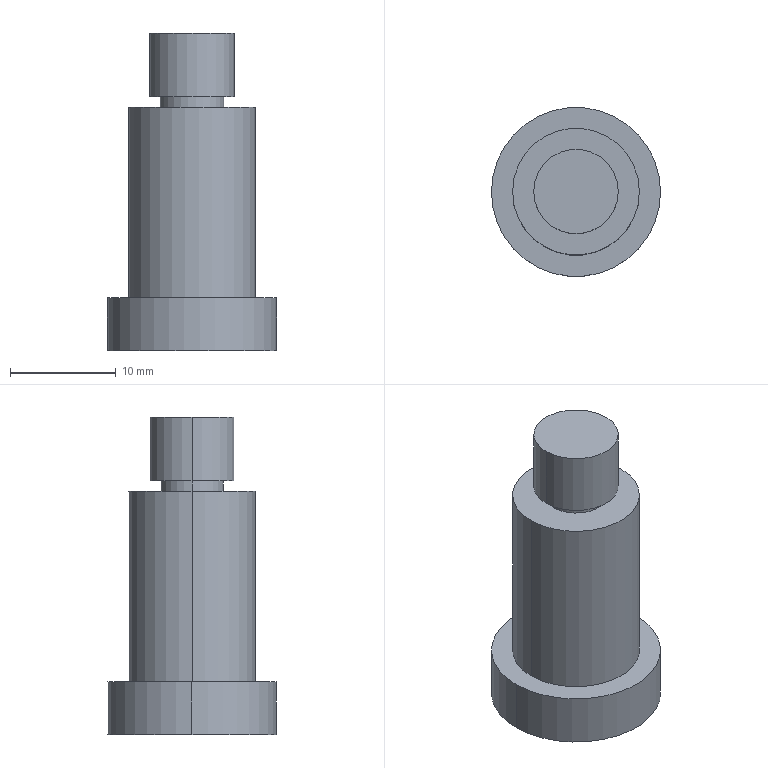Part | SolidWorks | features Revolution 1 | 1 solid | 13 faces | box 16 x 16 x 30 mm | volume 3371 mm3 | cylinder 8 | plane 5 | commonest cylinder face diameters 6 x2 8 x2 12 x2 16 x2
STEP:
#1=CARTESIAN_POINT('',(4.,0.,-6.));
#2=VERTEX_POINT('',#1);
#3=CARTESIAN_POINT('',(-4.,0.,-6.));
#4=VERTEX_POINT('',#3);
#5=CARTESIAN_POINT('',(0.,0.,-6.));
#6=DIRECTION('',(0.,0.,1.));
#7=DIRECTION('',(1.,0.,0.));
#8=AXIS2_PLACEMENT_3D('',#5,#6,#7);
#9=CIRCLE('',#8,4.);
#10=EDGE_CURVE('',#2,#4,#9,.T.);
#11=ORIENTED_EDGE('',*,*,#10,.T.);
#12=CARTESIAN_POINT('',(-4.,0.,0.));
#13=VERTEX_POINT('',#12);
#14=CARTESIAN_POINT('',(-4.,0.,0.));
#15=DIRECTION('',(0.,0.,1.));
#16=VECTOR('',#15,1000.);
#17=LINE('',#14,#16);
#18=EDGE_CURVE('',#4,#13,#17,.T.);
#19=ORIENTED_EDGE('',*,*,#18,.T.);
#20=CARTESIAN_POINT('',(4.,0.,0.));
#21=VERTEX_POINT('',#20);
#22=CARTESIAN_POINT('',(0.,0.,0.));
#23=DIRECTION('',(0.,0.,1.));
#24=DIRECTION('',(1.,0.,0.));
#25=AXIS2_PLACEMENT_3D('',#22,#23,#24);
#26=CIRCLE('',#25,4.);
#27=EDGE_CURVE('',#21,#13,#26,.T.);
#28=ORIENTED_EDGE('',*,*,#27,.F.);
#29=CARTESIAN_POINT('',(4.,0.,0.));
#30=DIRECTION('',(0.,0.,1.));
#31=VECTOR('',#30,1000.);
#32=LINE('',#29,#31);
#33=EDGE_CURVE('',#2,#21,#32,.T.);
#34=ORIENTED_EDGE('',*,*,#33,.F.);
#35=EDGE_LOOP('',(#11,#19,#28,#34));
#36=FACE_OUTER_BOUND('',#35,.T.);
#37=CARTESIAN_POINT('',(0.,0.,0.));
#38=DIRECTION('',(0.,0.,1.));
#39=DIRECTION('',(1.,0.,0.));
#40=AXIS2_PLACEMENT_3D('',#37,#38,#39);
#41=CYLINDRICAL_SURFACE('',#40,4.);
#42=ADVANCED_FACE('',(#36),#41,.T.);
#43=CARTESIAN_POINT('',(3.,0.,-7.));
#44=VERTEX_POINT('',#43);
#45=CARTESIAN_POINT('',(-3.,0.,-7.));
#46=VERTEX_POINT('',#45);
#47=CARTESIAN_POINT('',(0.,0.,-7.));
#48=DIRECTION('',(0.,0.,1.));
#49=DIRECTION('',(1.,0.,0.));
#50=AXIS2_PLACEMENT_3D('',#47,#48,#49);
#51=CIRCLE('',#50,3.);
#52=EDGE_CURVE('',#44,#46,#51,.T.);
#53=ORIENTED_EDGE('',*,*,#52,.T.);
#54=CARTESIAN_POINT('',(-3.,0.,-6.));
#55=VERTEX_POINT('',#54);
#56=CARTESIAN_POINT('',(-3.,0.,0.));
#57=DIRECTION('',(0.,0.,1.));
#58=VECTOR('',#57,1000.);
#59=LINE('',#56,#58);
#60=EDGE_CURVE('',#46,#55,#59,.T.);
#61=ORIENTED_EDGE('',*,*,#60,.T.);
#62=CARTESIAN_POINT('',(3.,0.,-6.));
#63=VERTEX_POINT('',#62);
#64=CARTESIAN_POINT('',(0.,0.,-6.));
#65=DIRECTION('',(0.,0.,1.));
#66=DIRECTION('',(1.,0.,0.));
#67=AXIS2_PLACEMENT_3D('',#64,#65,#66);
#68=CIRCLE('',#67,3.);
#69=EDGE_CURVE('',#63,#55,#68,.T.);
#70=ORIENTED_EDGE('',*,*,#69,.F.);
#71=CARTESIAN_POINT('',(3.,0.,0.));
#72=DIRECTION('',(0.,0.,1.));
#73=VECTOR('',#72,1000.);
#74=LINE('',#71,#73);
#75=EDGE_CURVE('',#44,#63,#74,.T.);
#76=ORIENTED_EDGE('',*,*,#75,.F.);
#77=EDGE_LOOP('',(#53,#61,#70,#76));
#78=FACE_OUTER_BOUND('',#77,.T.);
#79=CARTESIAN_POINT('',(0.,0.,0.));
#80=DIRECTION('',(0.,0.,1.));
#81=DIRECTION('',(1.,0.,0.));
#82=AXIS2_PLACEMENT_3D('',#79,#80,#81);
#83=CYLINDRICAL_SURFACE('',#82,3.);
#84=ADVANCED_FACE('',(#78),#83,.T.);
#85=CARTESIAN_POINT('',(6.,0.,-25.));
#86=VERTEX_POINT('',#85);
#87=CARTESIAN_POINT('',(-6.,0.,-25.));
#88=VERTEX_POINT('',#87);
#89=CARTESIAN_POINT('',(0.,0.,-25.));
#90=DIRECTION('',(0.,0.,1.));
#91=DIRECTION('',(1.,0.,0.));
#92=AXIS2_PLACEMENT_3D('',#89,#90,#91);
#93=CIRCLE('',#92,6.);
#94=EDGE_CURVE('',#86,#88,#93,.T.);
#95=ORIENTED_EDGE('',*,*,#94,.T.);
#96=CARTESIAN_POINT('',(-6.,0.,-7.));
#97=VERTEX_POINT('',#96);
#98=CARTESIAN_POINT('',(-6.,0.,0.));
#99=DIRECTION('',(0.,0.,1.));
#100=VECTOR('',#99,1000.);
#101=LINE('',#98,#100);
#102=EDGE_CURVE('',#88,#97,#101,.T.);
#103=ORIENTED_EDGE('',*,*,#102,.T.);
#104=CARTESIAN_POINT('',(6.,0.,-7.));
#105=VERTEX_POINT('',#104);
#106=CARTESIAN_POINT('',(0.,0.,-7.));
#107=DIRECTION('',(0.,0.,1.));
#108=DIRECTION('',(1.,0.,0.));
#109=AXIS2_PLACEMENT_3D('',#106,#107,#108);
#110=CIRCLE('',#109,6.);
#111=EDGE_CURVE('',#105,#97,#110,.T.);
#112=ORIENTED_EDGE('',*,*,#111,.F.);
#113=CARTESIAN_POINT('',(6.,0.,0.));
#114=DIRECTION('',(0.,0.,1.));
#115=VECTOR('',#114,1000.);
#116=LINE('',#113,#115);
#117=EDGE_CURVE('',#86,#105,#116,.T.);
#118=ORIENTED_EDGE('',*,*,#117,.F.);
#119=EDGE_LOOP('',(#95,#103,#112,#118));
#120=FACE_OUTER_BOUND('',#119,.T.);
#121=CARTESIAN_POINT('',(0.,0.,0.));
#122=DIRECTION('',(0.,0.,1.));
#123=DIRECTION('',(1.,0.,0.));
#124=AXIS2_PLACEMENT_3D('',#121,#122,#123);
#125=CYLINDRICAL_SURFACE('',#124,6.);
#126=ADVANCED_FACE('',(#120),#125,.T.);
#127=CARTESIAN_POINT('',(8.,0.,-30.));
#128=VERTEX_POINT('',#127);
#129=CARTESIAN_POINT('',(-8.,0.,-30.));
#130=VERTEX_POINT('',#129);
#131=CARTESIAN_POINT('',(0.,0.,-30.));
#132=DIRECTION('',(0.,0.,1.));
#133=DIRECTION('',(1.,0.,0.));
#134=AXIS2_PLACEMENT_3D('',#131,#132,#133);
#135=CIRCLE('',#134,8.);
#136=EDGE_CURVE('',#128,#130,#135,.T.);
#137=ORIENTED_EDGE('',*,*,#136,.T.);
#138=CARTESIAN_POINT('',(-8.,0.,-25.));
#139=VERTEX_POINT('',#138);
#140=CARTESIAN_POINT('',(-8.,0.,0.));
#141=DIRECTION('',(0.,0.,1.));
#142=VECTOR('',#141,1000.);
#143=LINE('',#140,#142);
#144=EDGE_CURVE('',#130,#139,#143,.T.);
#145=ORIENTED_EDGE('',*,*,#144,.T.);
#146=CARTESIAN_POINT('',(8.,0.,-25.));
#147=VERTEX_POINT('',#146);
#148=CARTESIAN_POINT('',(0.,0.,-25.));
#149=DIRECTION('',(0.,0.,1.));
#150=DIRECTION('',(1.,0.,0.));
#151=AXIS2_PLACEMENT_3D('',#148,#149,#150);
#152=CIRCLE('',#151,8.);
#153=EDGE_CURVE('',#147,#139,#152,.T.);
#154=ORIENTED_EDGE('',*,*,#153,.F.);
#155=CARTESIAN_POINT('',(8.,0.,0.));
#156=DIRECTION('',(0.,0.,1.));
#157=VECTOR('',#156,1000.);
#158=LINE('',#155,#157);
#159=EDGE_CURVE('',#128,#147,#158,.T.);
#160=ORIENTED_EDGE('',*,*,#159,.F.);
#161=EDGE_LOOP('',(#137,#145,#154,#160));
#162=FACE_OUTER_BOUND('',#161,.T.);
#163=CARTESIAN_POINT('',(0.,0.,0.));
#164=DIRECTION('',(0.,0.,1.));
#165=DIRECTION('',(1.,0.,0.));
#166=AXIS2_PLACEMENT_3D('',#163,#164,#165);
#167=CYLINDRICAL_SURFACE('',#166,8.);
#168=ADVANCED_FACE('',(#162),#167,.T.);
#169=ORIENTED_EDGE('',*,*,#136,.F.);
#170=CARTESIAN_POINT('',(0.,0.,-30.));
#171=DIRECTION('',(0.,0.,1.));
#172=DIRECTION('',(1.,0.,0.));
#173=AXIS2_PLACEMENT_3D('',#170,#171,#172);
#174=CIRCLE('',#173,8.);
#175=EDGE_CURVE('',#130,#128,#174,.T.);
#176=ORIENTED_EDGE('',*,*,#175,.F.);
#177=EDGE_LOOP('',(#169,#176));
#178=FACE_OUTER_BOUND('',#177,.T.);
#179=CARTESIAN_POINT('',(0.,0.,-30.));
#180=DIRECTION('',(0.,0.,1.));
#181=DIRECTION('',(1.,0.,0.));
#182=AXIS2_PLACEMENT_3D('',#179,#180,#181);
#183=PLANE('',#182);
#184=ADVANCED_FACE('',(#178),#183,.F.);
#185=ORIENTED_EDGE('',*,*,#144,.F.);
#186=ORIENTED_EDGE('',*,*,#175,.T.);
#187=ORIENTED_EDGE('',*,*,#159,.T.);
#188=CARTESIAN_POINT('',(0.,0.,-25.));
#189=DIRECTION('',(0.,0.,1.));
#190=DIRECTION('',(1.,0.,0.));
#191=AXIS2_PLACEMENT_3D('',#188,#189,#190);
#192=CIRCLE('',#191,8.);
#193=EDGE_CURVE('',#139,#147,#192,.T.);
#194=ORIENTED_EDGE('',*,*,#193,.F.);
#195=EDGE_LOOP('',(#185,#186,#187,#194));
#196=FACE_OUTER_BOUND('',#195,.T.);
#197=CARTESIAN_POINT('',(0.,0.,0.));
#198=DIRECTION('',(0.,0.,1.));
#199=DIRECTION('',(1.,0.,0.));
#200=AXIS2_PLACEMENT_3D('',#197,#198,#199);
#201=CYLINDRICAL_SURFACE('',#200,8.);
#202=ADVANCED_FACE('',(#196),#201,.T.);
#203=ORIENTED_EDGE('',*,*,#94,.F.);
#204=CARTESIAN_POINT('',(0.,0.,-25.));
#205=DIRECTION('',(0.,0.,1.));
#206=DIRECTION('',(1.,0.,0.));
#207=AXIS2_PLACEMENT_3D('',#204,#205,#206);
#208=CIRCLE('',#207,6.);
#209=EDGE_CURVE('',#88,#86,#208,.T.);
#210=ORIENTED_EDGE('',*,*,#209,.F.);
#211=EDGE_LOOP('',(#203,#210));
#212=FACE_BOUND('',#211,.T.);
#213=ORIENTED_EDGE('',*,*,#153,.T.);
#214=ORIENTED_EDGE('',*,*,#193,.T.);
#215=EDGE_LOOP('',(#213,#214));
#216=FACE_OUTER_BOUND('',#215,.T.);
#217=CARTESIAN_POINT('',(0.,8.,-25.));
#218=DIRECTION('',(0.,0.,-1.));
#219=DIRECTION('',(-1.,0.,0.));
#220=AXIS2_PLACEMENT_3D('',#217,#218,#219);
#221=PLANE('',#220);
#222=ADVANCED_FACE('',(#212,#216),#221,.F.);
#223=ORIENTED_EDGE('',*,*,#102,.F.);
#224=ORIENTED_EDGE('',*,*,#209,.T.);
#225=ORIENTED_EDGE('',*,*,#117,.T.);
#226=CARTESIAN_POINT('',(0.,0.,-7.));
#227=DIRECTION('',(0.,0.,1.));
#228=DIRECTION('',(1.,0.,0.));
#229=AXIS2_PLACEMENT_3D('',#226,#227,#228);
#230=CIRCLE('',#229,6.);
#231=EDGE_CURVE('',#97,#105,#230,.T.);
#232=ORIENTED_EDGE('',*,*,#231,.F.);
#233=EDGE_LOOP('',(#223,#224,#225,#232));
#234=FACE_OUTER_BOUND('',#233,.T.);
#235=CARTESIAN_POINT('',(0.,0.,0.));
#236=DIRECTION('',(0.,0.,1.));
#237=DIRECTION('',(1.,0.,0.));
#238=AXIS2_PLACEMENT_3D('',#235,#236,#237);
#239=CYLINDRICAL_SURFACE('',#238,6.);
#240=ADVANCED_FACE('',(#234),#239,.T.);
#241=ORIENTED_EDGE('',*,*,#52,.F.);
#242=CARTESIAN_POINT('',(0.,0.,-7.));
#243=DIRECTION('',(0.,0.,1.));
#244=DIRECTION('',(1.,0.,0.));
#245=AXIS2_PLACEMENT_3D('',#242,#243,#244);
#246=CIRCLE('',#245,3.);
#247=EDGE_CURVE('',#46,#44,#246,.T.);
#248=ORIENTED_EDGE('',*,*,#247,.F.);
#249=EDGE_LOOP('',(#241,#248));
#250=FACE_BOUND('',#249,.T.);
#251=ORIENTED_EDGE('',*,*,#111,.T.);
#252=ORIENTED_EDGE('',*,*,#231,.T.);
#253=EDGE_LOOP('',(#251,#252));
#254=FACE_OUTER_BOUND('',#253,.T.);
#255=CARTESIAN_POINT('',(0.,6.,-7.));
#256=DIRECTION('',(0.,0.,-1.));
#257=DIRECTION('',(-1.,0.,0.));
#258=AXIS2_PLACEMENT_3D('',#255,#256,#257);
#259=PLANE('',#258);
#260=ADVANCED_FACE('',(#250,#254),#259,.F.);
#261=ORIENTED_EDGE('',*,*,#60,.F.);
#262=ORIENTED_EDGE('',*,*,#247,.T.);
#263=ORIENTED_EDGE('',*,*,#75,.T.);
#264=CARTESIAN_POINT('',(0.,0.,-6.));
#265=DIRECTION('',(0.,0.,1.));
#266=DIRECTION('',(1.,0.,0.));
#267=AXIS2_PLACEMENT_3D('',#264,#265,#266);
#268=CIRCLE('',#267,3.);
#269=EDGE_CURVE('',#55,#63,#268,.T.);
#270=ORIENTED_EDGE('',*,*,#269,.F.);
#271=EDGE_LOOP('',(#261,#262,#263,#270));
#272=FACE_OUTER_BOUND('',#271,.T.);
#273=CARTESIAN_POINT('',(0.,0.,0.));
#274=DIRECTION('',(0.,0.,1.));
#275=DIRECTION('',(1.,0.,0.));
#276=AXIS2_PLACEMENT_3D('',#273,#274,#275);
#277=CYLINDRICAL_SURFACE('',#276,3.);
#278=ADVANCED_FACE('',(#272),#277,.T.);
#279=ORIENTED_EDGE('',*,*,#10,.F.);
#280=CARTESIAN_POINT('',(0.,0.,-6.));
#281=DIRECTION('',(0.,0.,1.));
#282=DIRECTION('',(1.,0.,0.));
#283=AXIS2_PLACEMENT_3D('',#280,#281,#282);
#284=CIRCLE('',#283,4.);
#285=EDGE_CURVE('',#4,#2,#284,.T.);
#286=ORIENTED_EDGE('',*,*,#285,.F.);
#287=EDGE_LOOP('',(#279,#286));
#288=FACE_OUTER_BOUND('',#287,.T.);
#289=ORIENTED_EDGE('',*,*,#69,.T.);
#290=ORIENTED_EDGE('',*,*,#269,.T.);
#291=EDGE_LOOP('',(#289,#290));
#292=FACE_BOUND('',#291,.T.);
#293=CARTESIAN_POINT('',(0.,3.,-6.));
#294=DIRECTION('',(0.,0.,1.));
#295=DIRECTION('',(1.,0.,0.));
#296=AXIS2_PLACEMENT_3D('',#293,#294,#295);
#297=PLANE('',#296);
#298=ADVANCED_FACE('',(#288,#292),#297,.F.);
#299=ORIENTED_EDGE('',*,*,#18,.F.);
#300=ORIENTED_EDGE('',*,*,#285,.T.);
#301=ORIENTED_EDGE('',*,*,#33,.T.);
#302=CARTESIAN_POINT('',(0.,0.,0.));
#303=DIRECTION('',(0.,0.,1.));
#304=DIRECTION('',(1.,0.,0.));
#305=AXIS2_PLACEMENT_3D('',#302,#303,#304);
#306=CIRCLE('',#305,4.);
#307=EDGE_CURVE('',#13,#21,#306,.T.);
#308=ORIENTED_EDGE('',*,*,#307,.F.);
#309=EDGE_LOOP('',(#299,#300,#301,#308));
#310=FACE_OUTER_BOUND('',#309,.T.);
#311=CARTESIAN_POINT('',(0.,0.,0.));
#312=DIRECTION('',(0.,0.,1.));
#313=DIRECTION('',(1.,0.,0.));
#314=AXIS2_PLACEMENT_3D('',#311,#312,#313);
#315=CYLINDRICAL_SURFACE('',#314,4.);
#316=ADVANCED_FACE('',(#310),#315,.T.);
#317=ORIENTED_EDGE('',*,*,#27,.T.);
#318=ORIENTED_EDGE('',*,*,#307,.T.);
#319=EDGE_LOOP('',(#317,#318));
#320=FACE_OUTER_BOUND('',#319,.T.);
#321=CARTESIAN_POINT('',(0.,4.,0.));
#322=DIRECTION('',(0.,0.,-1.));
#323=DIRECTION('',(-1.,0.,0.));
#324=AXIS2_PLACEMENT_3D('',#321,#322,#323);
#325=PLANE('',#324);
#326=ADVANCED_FACE('',(#320),#325,.F.);
#327=CLOSED_SHELL('',(#42,#84,#126,#168,#184,#202,#222,#240,#260,#278,#298,#316,#326));
#328=MANIFOLD_SOLID_BREP('',#327);
#329=CARTESIAN_POINT('',(0.,0.,0.));
#330=DIRECTION('',(0.,0.,1.));
#331=DIRECTION('',(1.,0.,0.));
#332=AXIS2_PLACEMENT_3D('',#329,#330,#331);
#333=(LENGTH_UNIT()NAMED_UNIT(*)SI_UNIT(.MILLI.,.METRE.));
#334=UNCERTAINTY_MEASURE_WITH_UNIT(LENGTH_MEASURE(0.00001),#333,'','');
#335=(NAMED_UNIT(*)PLANE_ANGLE_UNIT()SI_UNIT($,.RADIAN.));
#336=(NAMED_UNIT(*)SI_UNIT($,.STERADIAN.)SOLID_ANGLE_UNIT());
#337=(GEOMETRIC_REPRESENTATION_CONTEXT(3)GLOBAL_UNCERTAINTY_ASSIGNED_CONTEXT((#334))GLOBAL_UNIT_ASSIGNED_CONTEXT((#333,#335,#336))REPRESENTATION_CONTEXT('',''));
#338=ADVANCED_BREP_SHAPE_REPRESENTATION('',(#328,#332),#337);